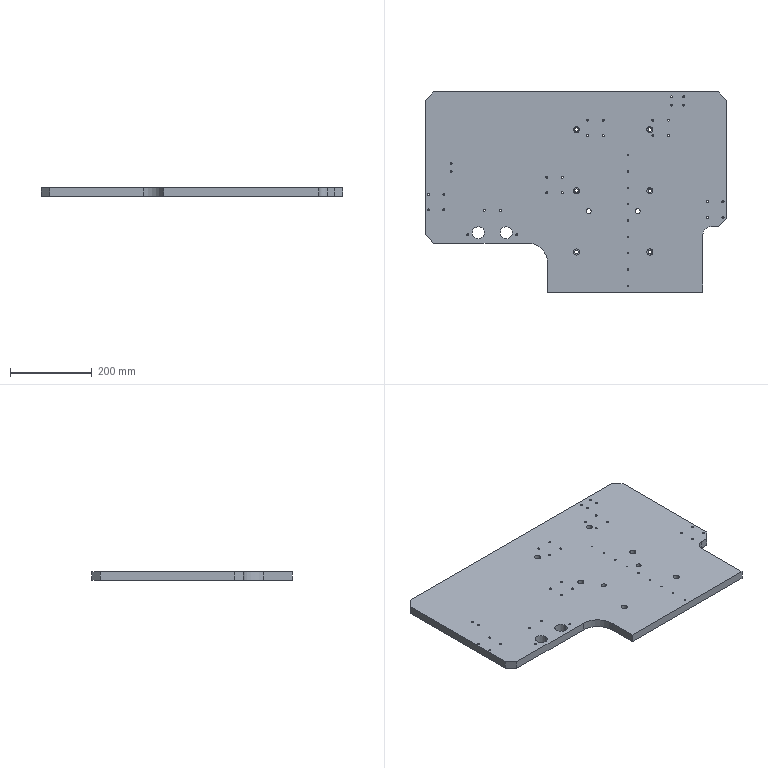Part | SolidWorks | features HoleWzd 6, Cut 4, Chamfer 2, Extrusion 1 | 1 solid | 132 faces | box 738 x 490 x 20 mm | volume 6263387 mm3 | cylinder 112 | plane 20 | commonest cylinder face diameters 5 x60 3.3 x18 9 x12 15 x12 12 x4 30 x4